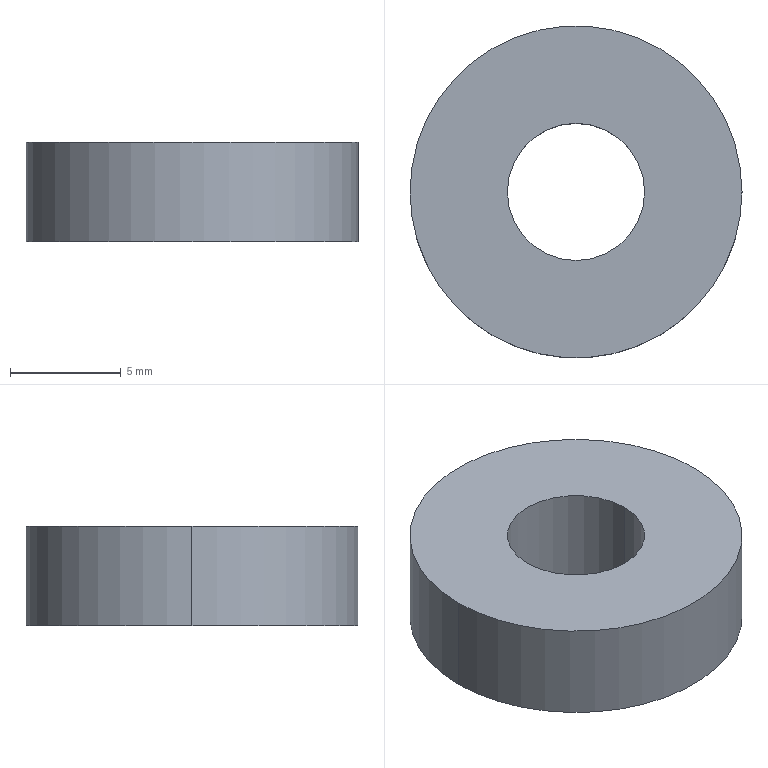Part | SolidWorks | features FlatPattern 1, SMBaseFlange 1, SheetMetal 1 | 1 solid | 6 faces | box 15 x 15 x 4.5 mm | volume 659.357 mm3 | cylinder 4 | plane 2 | commonest cylinder face diameters 6.2 x2 15 x2
STEP:
#1=CARTESIAN_POINT('',(-3.1,0.,4.5));
#2=VERTEX_POINT('',#1);
#3=CARTESIAN_POINT('',(3.1,0.,4.5));
#4=VERTEX_POINT('',#3);
#5=CARTESIAN_POINT('',(0.,0.,4.5));
#6=DIRECTION('',(0.,0.,1.));
#7=DIRECTION('',(1.,0.,0.));
#8=AXIS2_PLACEMENT_3D('',#5,#6,#7);
#9=CIRCLE('',#8,3.1);
#10=EDGE_CURVE('',#2,#4,#9,.T.);
#11=ORIENTED_EDGE('',*,*,#10,.T.);
#12=CARTESIAN_POINT('',(3.1,0.,0.));
#13=VERTEX_POINT('',#12);
#14=CARTESIAN_POINT('',(3.1,0.,4.5));
#15=DIRECTION('',(0.,0.,-1.));
#16=VECTOR('',#15,1000.);
#17=LINE('',#14,#16);
#18=EDGE_CURVE('',#4,#13,#17,.T.);
#19=ORIENTED_EDGE('',*,*,#18,.T.);
#20=CARTESIAN_POINT('',(-3.1,0.,0.));
#21=VERTEX_POINT('',#20);
#22=CARTESIAN_POINT('',(0.,0.,0.));
#23=DIRECTION('',(0.,0.,1.));
#24=DIRECTION('',(1.,0.,0.));
#25=AXIS2_PLACEMENT_3D('',#22,#23,#24);
#26=CIRCLE('',#25,3.1);
#27=EDGE_CURVE('',#21,#13,#26,.T.);
#28=ORIENTED_EDGE('',*,*,#27,.F.);
#29=CARTESIAN_POINT('',(-3.1,0.,4.5));
#30=DIRECTION('',(0.,0.,-1.));
#31=VECTOR('',#30,1000.);
#32=LINE('',#29,#31);
#33=EDGE_CURVE('',#2,#21,#32,.T.);
#34=ORIENTED_EDGE('',*,*,#33,.F.);
#35=EDGE_LOOP('',(#11,#19,#28,#34));
#36=FACE_OUTER_BOUND('',#35,.T.);
#37=CARTESIAN_POINT('',(0.,0.,4.5));
#38=DIRECTION('',(0.,0.,-1.));
#39=DIRECTION('',(-1.,0.,0.));
#40=AXIS2_PLACEMENT_3D('',#37,#38,#39);
#41=CYLINDRICAL_SURFACE('',#40,3.1);
#42=ADVANCED_FACE('',(#36),#41,.F.);
#43=CARTESIAN_POINT('',(7.5,0.,4.5));
#44=VERTEX_POINT('',#43);
#45=CARTESIAN_POINT('',(-7.5,0.,4.5));
#46=VERTEX_POINT('',#45);
#47=CARTESIAN_POINT('',(0.,0.,4.5));
#48=DIRECTION('',(0.,0.,1.));
#49=DIRECTION('',(1.,0.,0.));
#50=AXIS2_PLACEMENT_3D('',#47,#48,#49);
#51=CIRCLE('',#50,7.5);
#52=EDGE_CURVE('',#44,#46,#51,.T.);
#53=ORIENTED_EDGE('',*,*,#52,.F.);
#54=CARTESIAN_POINT('',(7.5,0.,0.));
#55=VERTEX_POINT('',#54);
#56=CARTESIAN_POINT('',(7.5,0.,4.5));
#57=DIRECTION('',(0.,0.,-1.));
#58=VECTOR('',#57,1000.);
#59=LINE('',#56,#58);
#60=EDGE_CURVE('',#44,#55,#59,.T.);
#61=ORIENTED_EDGE('',*,*,#60,.T.);
#62=CARTESIAN_POINT('',(-7.5,0.,0.));
#63=VERTEX_POINT('',#62);
#64=CARTESIAN_POINT('',(0.,0.,0.));
#65=DIRECTION('',(0.,0.,1.));
#66=DIRECTION('',(1.,0.,0.));
#67=AXIS2_PLACEMENT_3D('',#64,#65,#66);
#68=CIRCLE('',#67,7.5);
#69=EDGE_CURVE('',#55,#63,#68,.T.);
#70=ORIENTED_EDGE('',*,*,#69,.T.);
#71=CARTESIAN_POINT('',(-7.5,0.,4.5));
#72=DIRECTION('',(0.,0.,-1.));
#73=VECTOR('',#72,1000.);
#74=LINE('',#71,#73);
#75=EDGE_CURVE('',#46,#63,#74,.T.);
#76=ORIENTED_EDGE('',*,*,#75,.F.);
#77=EDGE_LOOP('',(#53,#61,#70,#76));
#78=FACE_OUTER_BOUND('',#77,.T.);
#79=CARTESIAN_POINT('',(0.,0.,4.5));
#80=DIRECTION('',(0.,0.,-1.));
#81=DIRECTION('',(-1.,0.,0.));
#82=AXIS2_PLACEMENT_3D('',#79,#80,#81);
#83=CYLINDRICAL_SURFACE('',#82,7.5);
#84=ADVANCED_FACE('',(#78),#83,.T.);
#85=CARTESIAN_POINT('',(0.,0.,4.5));
#86=DIRECTION('',(0.,0.,1.));
#87=DIRECTION('',(1.,0.,0.));
#88=AXIS2_PLACEMENT_3D('',#85,#86,#87);
#89=CIRCLE('',#88,7.5);
#90=EDGE_CURVE('',#46,#44,#89,.T.);
#91=ORIENTED_EDGE('',*,*,#90,.T.);
#92=ORIENTED_EDGE('',*,*,#52,.T.);
#93=EDGE_LOOP('',(#91,#92));
#94=FACE_OUTER_BOUND('',#93,.T.);
#95=ORIENTED_EDGE('',*,*,#10,.F.);
#96=CARTESIAN_POINT('',(0.,0.,4.5));
#97=DIRECTION('',(0.,0.,1.));
#98=DIRECTION('',(1.,0.,0.));
#99=AXIS2_PLACEMENT_3D('',#96,#97,#98);
#100=CIRCLE('',#99,3.1);
#101=EDGE_CURVE('',#4,#2,#100,.T.);
#102=ORIENTED_EDGE('',*,*,#101,.F.);
#103=EDGE_LOOP('',(#95,#102));
#104=FACE_BOUND('',#103,.T.);
#105=CARTESIAN_POINT('',(0.,0.,4.5));
#106=DIRECTION('',(0.,0.,1.));
#107=DIRECTION('',(1.,0.,0.));
#108=AXIS2_PLACEMENT_3D('',#105,#106,#107);
#109=PLANE('',#108);
#110=ADVANCED_FACE('',(#94,#104),#109,.T.);
#111=CARTESIAN_POINT('',(0.,0.,0.));
#112=DIRECTION('',(0.,0.,1.));
#113=DIRECTION('',(1.,0.,0.));
#114=AXIS2_PLACEMENT_3D('',#111,#112,#113);
#115=CIRCLE('',#114,7.5);
#116=EDGE_CURVE('',#63,#55,#115,.T.);
#117=ORIENTED_EDGE('',*,*,#116,.F.);
#118=ORIENTED_EDGE('',*,*,#69,.F.);
#119=EDGE_LOOP('',(#117,#118));
#120=FACE_OUTER_BOUND('',#119,.T.);
#121=ORIENTED_EDGE('',*,*,#27,.T.);
#122=CARTESIAN_POINT('',(0.,0.,0.));
#123=DIRECTION('',(0.,0.,1.));
#124=DIRECTION('',(1.,0.,0.));
#125=AXIS2_PLACEMENT_3D('',#122,#123,#124);
#126=CIRCLE('',#125,3.1);
#127=EDGE_CURVE('',#13,#21,#126,.T.);
#128=ORIENTED_EDGE('',*,*,#127,.T.);
#129=EDGE_LOOP('',(#121,#128));
#130=FACE_BOUND('',#129,.T.);
#131=CARTESIAN_POINT('',(0.,0.,0.));
#132=DIRECTION('',(0.,0.,1.));
#133=DIRECTION('',(1.,0.,0.));
#134=AXIS2_PLACEMENT_3D('',#131,#132,#133);
#135=PLANE('',#134);
#136=ADVANCED_FACE('',(#120,#130),#135,.F.);
#137=ORIENTED_EDGE('',*,*,#60,.F.);
#138=ORIENTED_EDGE('',*,*,#90,.F.);
#139=ORIENTED_EDGE('',*,*,#75,.T.);
#140=ORIENTED_EDGE('',*,*,#116,.T.);
#141=EDGE_LOOP('',(#137,#138,#139,#140));
#142=FACE_OUTER_BOUND('',#141,.T.);
#143=CARTESIAN_POINT('',(0.,0.,4.5));
#144=DIRECTION('',(0.,0.,-1.));
#145=DIRECTION('',(-1.,0.,0.));
#146=AXIS2_PLACEMENT_3D('',#143,#144,#145);
#147=CYLINDRICAL_SURFACE('',#146,7.5);
#148=ADVANCED_FACE('',(#142),#147,.T.);
#149=ORIENTED_EDGE('',*,*,#18,.F.);
#150=ORIENTED_EDGE('',*,*,#101,.T.);
#151=ORIENTED_EDGE('',*,*,#33,.T.);
#152=ORIENTED_EDGE('',*,*,#127,.F.);
#153=EDGE_LOOP('',(#149,#150,#151,#152));
#154=FACE_OUTER_BOUND('',#153,.T.);
#155=CARTESIAN_POINT('',(0.,0.,4.5));
#156=DIRECTION('',(0.,0.,-1.));
#157=DIRECTION('',(-1.,0.,0.));
#158=AXIS2_PLACEMENT_3D('',#155,#156,#157);
#159=CYLINDRICAL_SURFACE('',#158,3.1);
#160=ADVANCED_FACE('',(#154),#159,.F.);
#161=CLOSED_SHELL('',(#42,#84,#110,#136,#148,#160));
#162=MANIFOLD_SOLID_BREP('',#161);
#163=CARTESIAN_POINT('',(0.,0.,0.));
#164=DIRECTION('',(0.,0.,1.));
#165=DIRECTION('',(1.,0.,0.));
#166=AXIS2_PLACEMENT_3D('',#163,#164,#165);
#167=(LENGTH_UNIT()NAMED_UNIT(*)SI_UNIT(.MILLI.,.METRE.));
#168=UNCERTAINTY_MEASURE_WITH_UNIT(LENGTH_MEASURE(0.00001),#167,'','');
#169=(NAMED_UNIT(*)PLANE_ANGLE_UNIT()SI_UNIT($,.RADIAN.));
#170=(NAMED_UNIT(*)SI_UNIT($,.STERADIAN.)SOLID_ANGLE_UNIT());
#171=(GEOMETRIC_REPRESENTATION_CONTEXT(3)GLOBAL_UNCERTAINTY_ASSIGNED_CONTEXT((#168))GLOBAL_UNIT_ASSIGNED_CONTEXT((#167,#169,#170))REPRESENTATION_CONTEXT('',''));
#172=ADVANCED_BREP_SHAPE_REPRESENTATION('',(#162,#166),#171);